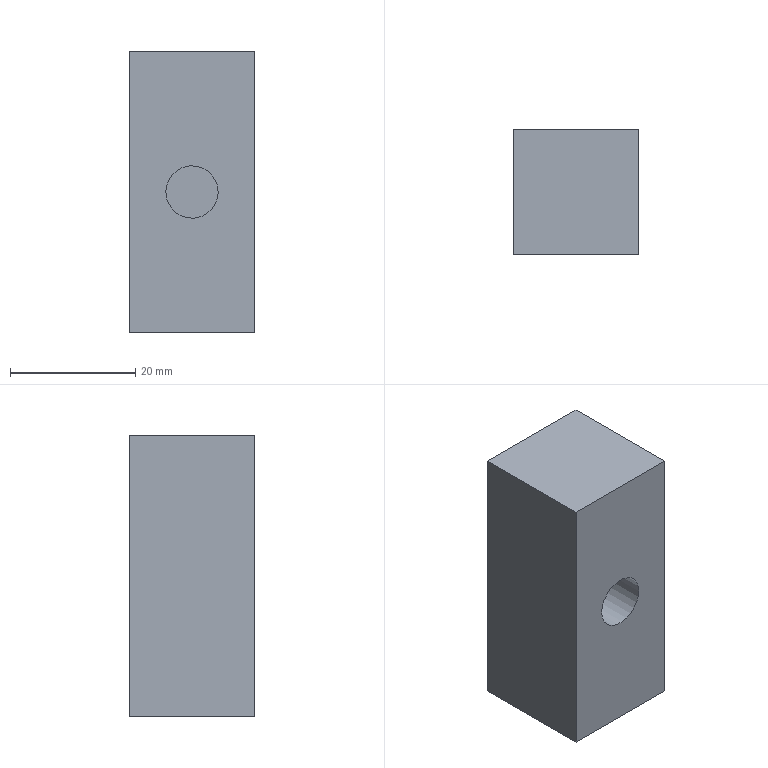Part | STEP file | SN10_017_001-02_BLOCO | 1 solid | 8 faces | box 20 x 20 x 45 mm | volume 17008 mm3 | plane 7 | cylinder 1 | commonest cylinder face diameters 8.376 x1
STEP:
#1=CARTESIAN_POINT('',(0.,0.,0.));
#2=DIRECTION('',(0.,0.,1.));
#3=DIRECTION('',(1.,0.,0.));
#4=AXIS2_PLACEMENT_3D('',#1,#2,#3);
#5=CARTESIAN_POINT('',(3876.675,-1747.,65.492));
#6=VERTEX_POINT('',#5);
#7=CARTESIAN_POINT('',(3873.,-1747.,67.5));
#8=DIRECTION('',(0.,1.,0.));
#9=DIRECTION('',(1.,0.,0.));
#10=AXIS2_PLACEMENT_3D('',#7,#8,#9);
#11=CIRCLE('',#10,4.188);
#12=CARTESIAN_POINT('',(3873.,-1747.,67.5));
#13=DIRECTION('',(0.,1.,0.));
#14=DIRECTION('',(0.,0.,1.));
#15=AXIS2_PLACEMENT_3D('',#12,#13,#14);
#16=PLANE('',#15);
#17=CARTESIAN_POINT('',(0.,0.));
#18=DIRECTION('',(0.,1.));
#19=AXIS2_PLACEMENT_2D('',#17,#18);
#20=CIRCLE('',#19,4.188);
#21=(GEOMETRIC_REPRESENTATION_CONTEXT(2)PARAMETRIC_REPRESENTATION_CONTEXT()REPRESENTATION_CONTEXT('',''));
#22=DEFINITIONAL_REPRESENTATION('',(#20),#21);
#23=PCURVE('',#16,#22);
#24=CARTESIAN_POINT('',(3873.,-1764.9,67.5));
#25=DIRECTION('',(0.,1.,0.));
#26=DIRECTION('',(0.8776,0.,-0.4794));
#27=AXIS2_PLACEMENT_3D('',#24,#25,#26);
#28=CYLINDRICAL_SURFACE('',#27,4.188);
#29=CARTESIAN_POINT('',(-0.5,17.9));
#30=DIRECTION('',(1.,0.));
#31=VECTOR('',#30,1.);
#32=LINE('',#29,#31);
#33=(GEOMETRIC_REPRESENTATION_CONTEXT(2)PARAMETRIC_REPRESENTATION_CONTEXT()REPRESENTATION_CONTEXT('',''));
#34=DEFINITIONAL_REPRESENTATION('',(#32),#33);
#35=PCURVE('',#28,#34);
#36=SURFACE_CURVE('',#11,(#23,#35),.PCURVE_S1.);
#37=EDGE_CURVE('',#6,#6,#36,.T.);
#38=ORIENTED_EDGE('',*,*,#37,.F.);
#39=EDGE_LOOP('',(#38));
#40=FACE_BOUND('',#39,.T.);
#41=ADVANCED_FACE('',(#40),#16,.F.);
#42=CARTESIAN_POINT('',(3883.,-1745.,90.));
#43=VERTEX_POINT('',#42);
#44=CARTESIAN_POINT('',(3863.,-1745.,90.));
#45=VERTEX_POINT('',#44);
#46=CARTESIAN_POINT('',(3883.,-1745.,90.));
#47=DIRECTION('',(-1.,0.,0.));
#48=VECTOR('',#47,1.);
#49=LINE('',#46,#48);
#50=CARTESIAN_POINT('',(0.,-1745.,0.));
#51=DIRECTION('',(0.,1.,0.));
#52=DIRECTION('',(0.,0.,1.));
#53=AXIS2_PLACEMENT_3D('',#50,#51,#52);
#54=PLANE('',#53);
#55=CARTESIAN_POINT('',(90.,3883.));
#56=DIRECTION('',(0.,-1.));
#57=VECTOR('',#56,1.);
#58=LINE('',#55,#57);
#59=(GEOMETRIC_REPRESENTATION_CONTEXT(2)PARAMETRIC_REPRESENTATION_CONTEXT()REPRESENTATION_CONTEXT('',''));
#60=DEFINITIONAL_REPRESENTATION('',(#58),#59);
#61=PCURVE('',#54,#60);
#62=CARTESIAN_POINT('',(3883.,-1745.,90.));
#63=DIRECTION('',(0.,0.,1.));
#64=DIRECTION('',(1.,0.,0.));
#65=AXIS2_PLACEMENT_3D('',#62,#63,#64);
#66=PLANE('',#65);
#67=CARTESIAN_POINT('',(0.,0.));
#68=DIRECTION('',(-1.,0.));
#69=VECTOR('',#68,1.);
#70=LINE('',#67,#69);
#71=(GEOMETRIC_REPRESENTATION_CONTEXT(2)PARAMETRIC_REPRESENTATION_CONTEXT()REPRESENTATION_CONTEXT('',''));
#72=DEFINITIONAL_REPRESENTATION('',(#70),#71);
#73=PCURVE('',#66,#72);
#74=SURFACE_CURVE('',#49,(#61,#73),.PCURVE_S1.);
#75=EDGE_CURVE('',#43,#45,#74,.T.);
#76=ORIENTED_EDGE('',*,*,#75,.F.);
#77=CARTESIAN_POINT('',(3883.,-1745.,45.));
#78=VERTEX_POINT('',#77);
#79=CARTESIAN_POINT('',(3883.,-1745.,45.));
#80=DIRECTION('',(0.,0.,1.));
#81=VECTOR('',#80,1.);
#82=LINE('',#79,#81);
#83=CARTESIAN_POINT('',(45.,3883.));
#84=DIRECTION('',(1.,0.));
#85=VECTOR('',#84,1.);
#86=LINE('',#83,#85);
#87=(GEOMETRIC_REPRESENTATION_CONTEXT(2)PARAMETRIC_REPRESENTATION_CONTEXT()REPRESENTATION_CONTEXT('',''));
#88=DEFINITIONAL_REPRESENTATION('',(#86),#87);
#89=PCURVE('',#54,#88);
#90=CARTESIAN_POINT('',(3883.,-1745.,45.));
#91=DIRECTION('',(1.,0.,0.));
#92=DIRECTION('',(0.,0.,-1.));
#93=AXIS2_PLACEMENT_3D('',#90,#91,#92);
#94=PLANE('',#93);
#95=CARTESIAN_POINT('',(0.,0.));
#96=DIRECTION('',(-1.,0.));
#97=VECTOR('',#96,1.);
#98=LINE('',#95,#97);
#99=(GEOMETRIC_REPRESENTATION_CONTEXT(2)PARAMETRIC_REPRESENTATION_CONTEXT()REPRESENTATION_CONTEXT('',''));
#100=DEFINITIONAL_REPRESENTATION('',(#98),#99);
#101=PCURVE('',#94,#100);
#102=SURFACE_CURVE('',#82,(#89,#101),.PCURVE_S1.);
#103=EDGE_CURVE('',#78,#43,#102,.T.);
#104=ORIENTED_EDGE('',*,*,#103,.F.);
#105=CARTESIAN_POINT('',(3863.,-1745.,45.));
#106=VERTEX_POINT('',#105);
#107=CARTESIAN_POINT('',(3863.,-1745.,45.));
#108=DIRECTION('',(1.,0.,0.));
#109=VECTOR('',#108,1.);
#110=LINE('',#107,#109);
#111=CARTESIAN_POINT('',(45.,3863.));
#112=DIRECTION('',(0.,1.));
#113=VECTOR('',#112,1.);
#114=LINE('',#111,#113);
#115=(GEOMETRIC_REPRESENTATION_CONTEXT(2)PARAMETRIC_REPRESENTATION_CONTEXT()REPRESENTATION_CONTEXT('',''));
#116=DEFINITIONAL_REPRESENTATION('',(#114),#115);
#117=PCURVE('',#54,#116);
#118=CARTESIAN_POINT('',(3863.,-1745.,45.));
#119=DIRECTION('',(0.,0.,-1.));
#120=DIRECTION('',(-1.,0.,0.));
#121=AXIS2_PLACEMENT_3D('',#118,#119,#120);
#122=PLANE('',#121);
#123=CARTESIAN_POINT('',(0.,0.));
#124=DIRECTION('',(-1.,0.));
#125=VECTOR('',#124,1.);
#126=LINE('',#123,#125);
#127=(GEOMETRIC_REPRESENTATION_CONTEXT(2)PARAMETRIC_REPRESENTATION_CONTEXT()REPRESENTATION_CONTEXT('',''));
#128=DEFINITIONAL_REPRESENTATION('',(#126),#127);
#129=PCURVE('',#122,#128);
#130=SURFACE_CURVE('',#110,(#117,#129),.PCURVE_S1.);
#131=EDGE_CURVE('',#106,#78,#130,.T.);
#132=ORIENTED_EDGE('',*,*,#131,.F.);
#133=CARTESIAN_POINT('',(3863.,-1745.,90.));
#134=DIRECTION('',(0.,0.,-1.));
#135=VECTOR('',#134,1.);
#136=LINE('',#133,#135);
#137=CARTESIAN_POINT('',(90.,3863.));
#138=DIRECTION('',(-1.,0.));
#139=VECTOR('',#138,1.);
#140=LINE('',#137,#139);
#141=(GEOMETRIC_REPRESENTATION_CONTEXT(2)PARAMETRIC_REPRESENTATION_CONTEXT()REPRESENTATION_CONTEXT('',''));
#142=DEFINITIONAL_REPRESENTATION('',(#140),#141);
#143=PCURVE('',#54,#142);
#144=CARTESIAN_POINT('',(3863.,-1745.,90.));
#145=DIRECTION('',(-1.,0.,0.));
#146=DIRECTION('',(0.,0.,1.));
#147=AXIS2_PLACEMENT_3D('',#144,#145,#146);
#148=PLANE('',#147);
#149=CARTESIAN_POINT('',(0.,0.));
#150=DIRECTION('',(-1.,0.));
#151=VECTOR('',#150,1.);
#152=LINE('',#149,#151);
#153=(GEOMETRIC_REPRESENTATION_CONTEXT(2)PARAMETRIC_REPRESENTATION_CONTEXT()REPRESENTATION_CONTEXT('',''));
#154=DEFINITIONAL_REPRESENTATION('',(#152),#153);
#155=PCURVE('',#148,#154);
#156=SURFACE_CURVE('',#136,(#143,#155),.PCURVE_S1.);
#157=EDGE_CURVE('',#45,#106,#156,.T.);
#158=ORIENTED_EDGE('',*,*,#157,.F.);
#159=EDGE_LOOP('',(#76,#104,#132,#158));
#160=FACE_BOUND('',#159,.T.);
#161=ADVANCED_FACE('',(#160),#54,.T.);
#162=CARTESIAN_POINT('',(3863.,-1765.,90.));
#163=VERTEX_POINT('',#162);
#164=CARTESIAN_POINT('',(3863.,-1765.,45.));
#165=VERTEX_POINT('',#164);
#166=CARTESIAN_POINT('',(3863.,-1765.,90.));
#167=DIRECTION('',(0.,0.,-1.));
#168=VECTOR('',#167,1.);
#169=LINE('',#166,#168);
#170=CARTESIAN_POINT('',(0.,-20.));
#171=DIRECTION('',(-1.,0.));
#172=VECTOR('',#171,1.);
#173=LINE('',#170,#172);
#174=(GEOMETRIC_REPRESENTATION_CONTEXT(2)PARAMETRIC_REPRESENTATION_CONTEXT()REPRESENTATION_CONTEXT('',''));
#175=DEFINITIONAL_REPRESENTATION('',(#173),#174);
#176=PCURVE('',#148,#175);
#177=CARTESIAN_POINT('',(0.,-1765.,0.));
#178=DIRECTION('',(0.,1.,0.));
#179=DIRECTION('',(0.,0.,1.));
#180=AXIS2_PLACEMENT_3D('',#177,#178,#179);
#181=PLANE('',#180);
#182=CARTESIAN_POINT('',(90.,3863.));
#183=DIRECTION('',(-1.,0.));
#184=VECTOR('',#183,1.);
#185=LINE('',#182,#184);
#186=(GEOMETRIC_REPRESENTATION_CONTEXT(2)PARAMETRIC_REPRESENTATION_CONTEXT()REPRESENTATION_CONTEXT('',''));
#187=DEFINITIONAL_REPRESENTATION('',(#185),#186);
#188=PCURVE('',#181,#187);
#189=SURFACE_CURVE('',#169,(#176,#188),.PCURVE_S1.);
#190=EDGE_CURVE('',#163,#165,#189,.T.);
#191=ORIENTED_EDGE('',*,*,#190,.F.);
#192=CARTESIAN_POINT('',(3863.,-1745.,90.));
#193=DIRECTION('',(0.,-1.,0.));
#194=VECTOR('',#193,1.);
#195=LINE('',#192,#194);
#196=CARTESIAN_POINT('',(0.,0.));
#197=DIRECTION('',(0.,-1.));
#198=VECTOR('',#197,1.);
#199=LINE('',#196,#198);
#200=(GEOMETRIC_REPRESENTATION_CONTEXT(2)PARAMETRIC_REPRESENTATION_CONTEXT()REPRESENTATION_CONTEXT('',''));
#201=DEFINITIONAL_REPRESENTATION('',(#199),#200);
#202=PCURVE('',#148,#201);
#203=CARTESIAN_POINT('',(-20.,0.));
#204=DIRECTION('',(0.,-1.));
#205=VECTOR('',#204,1.);
#206=LINE('',#203,#205);
#207=(GEOMETRIC_REPRESENTATION_CONTEXT(2)PARAMETRIC_REPRESENTATION_CONTEXT()REPRESENTATION_CONTEXT('',''));
#208=DEFINITIONAL_REPRESENTATION('',(#206),#207);
#209=PCURVE('',#66,#208);
#210=SURFACE_CURVE('',#195,(#202,#209),.PCURVE_S1.);
#211=EDGE_CURVE('',#45,#163,#210,.T.);
#212=ORIENTED_EDGE('',*,*,#211,.F.);
#213=ORIENTED_EDGE('',*,*,#157,.T.);
#214=CARTESIAN_POINT('',(3863.,-1745.,45.));
#215=DIRECTION('',(0.,-1.,0.));
#216=VECTOR('',#215,1.);
#217=LINE('',#214,#216);
#218=CARTESIAN_POINT('',(-45.,0.));
#219=DIRECTION('',(0.,-1.));
#220=VECTOR('',#219,1.);
#221=LINE('',#218,#220);
#222=(GEOMETRIC_REPRESENTATION_CONTEXT(2)PARAMETRIC_REPRESENTATION_CONTEXT()REPRESENTATION_CONTEXT('',''));
#223=DEFINITIONAL_REPRESENTATION('',(#221),#222);
#224=PCURVE('',#148,#223);
#225=CARTESIAN_POINT('',(0.,0.));
#226=DIRECTION('',(0.,-1.));
#227=VECTOR('',#226,1.);
#228=LINE('',#225,#227);
#229=(GEOMETRIC_REPRESENTATION_CONTEXT(2)PARAMETRIC_REPRESENTATION_CONTEXT()REPRESENTATION_CONTEXT('',''));
#230=DEFINITIONAL_REPRESENTATION('',(#228),#229);
#231=PCURVE('',#122,#230);
#232=SURFACE_CURVE('',#217,(#224,#231),.PCURVE_S1.);
#233=EDGE_CURVE('',#106,#165,#232,.T.);
#234=ORIENTED_EDGE('',*,*,#233,.T.);
#235=EDGE_LOOP('',(#191,#212,#213,#234));
#236=FACE_BOUND('',#235,.T.);
#237=ADVANCED_FACE('',(#236),#148,.T.);
#238=CARTESIAN_POINT('',(3883.,-1765.,45.));
#239=VERTEX_POINT('',#238);
#240=CARTESIAN_POINT('',(3863.,-1765.,45.));
#241=DIRECTION('',(1.,0.,0.));
#242=VECTOR('',#241,1.);
#243=LINE('',#240,#242);
#244=CARTESIAN_POINT('',(0.,-20.));
#245=DIRECTION('',(-1.,0.));
#246=VECTOR('',#245,1.);
#247=LINE('',#244,#246);
#248=(GEOMETRIC_REPRESENTATION_CONTEXT(2)PARAMETRIC_REPRESENTATION_CONTEXT()REPRESENTATION_CONTEXT('',''));
#249=DEFINITIONAL_REPRESENTATION('',(#247),#248);
#250=PCURVE('',#122,#249);
#251=CARTESIAN_POINT('',(45.,3863.));
#252=DIRECTION('',(0.,1.));
#253=VECTOR('',#252,1.);
#254=LINE('',#251,#253);
#255=(GEOMETRIC_REPRESENTATION_CONTEXT(2)PARAMETRIC_REPRESENTATION_CONTEXT()REPRESENTATION_CONTEXT('',''));
#256=DEFINITIONAL_REPRESENTATION('',(#254),#255);
#257=PCURVE('',#181,#256);
#258=SURFACE_CURVE('',#243,(#250,#257),.PCURVE_S1.);
#259=EDGE_CURVE('',#165,#239,#258,.T.);
#260=ORIENTED_EDGE('',*,*,#259,.F.);
#261=ORIENTED_EDGE('',*,*,#233,.F.);
#262=ORIENTED_EDGE('',*,*,#131,.T.);
#263=CARTESIAN_POINT('',(3883.,-1745.,45.));
#264=DIRECTION('',(0.,-1.,0.));
#265=VECTOR('',#264,1.);
#266=LINE('',#263,#265);
#267=CARTESIAN_POINT('',(-20.,0.));
#268=DIRECTION('',(0.,-1.));
#269=VECTOR('',#268,1.);
#270=LINE('',#267,#269);
#271=(GEOMETRIC_REPRESENTATION_CONTEXT(2)PARAMETRIC_REPRESENTATION_CONTEXT()REPRESENTATION_CONTEXT('',''));
#272=DEFINITIONAL_REPRESENTATION('',(#270),#271);
#273=PCURVE('',#122,#272);
#274=CARTESIAN_POINT('',(0.,0.));
#275=DIRECTION('',(0.,-1.));
#276=VECTOR('',#275,1.);
#277=LINE('',#274,#276);
#278=(GEOMETRIC_REPRESENTATION_CONTEXT(2)PARAMETRIC_REPRESENTATION_CONTEXT()REPRESENTATION_CONTEXT('',''));
#279=DEFINITIONAL_REPRESENTATION('',(#277),#278);
#280=PCURVE('',#94,#279);
#281=SURFACE_CURVE('',#266,(#273,#280),.PCURVE_S1.);
#282=EDGE_CURVE('',#78,#239,#281,.T.);
#283=ORIENTED_EDGE('',*,*,#282,.T.);
#284=EDGE_LOOP('',(#260,#261,#262,#283));
#285=FACE_BOUND('',#284,.T.);
#286=ADVANCED_FACE('',(#285),#122,.T.);
#287=CARTESIAN_POINT('',(3883.,-1765.,90.));
#288=VERTEX_POINT('',#287);
#289=CARTESIAN_POINT('',(3883.,-1765.,45.));
#290=DIRECTION('',(0.,0.,1.));
#291=VECTOR('',#290,1.);
#292=LINE('',#289,#291);
#293=CARTESIAN_POINT('',(0.,-20.));
#294=DIRECTION('',(-1.,0.));
#295=VECTOR('',#294,1.);
#296=LINE('',#293,#295);
#297=(GEOMETRIC_REPRESENTATION_CONTEXT(2)PARAMETRIC_REPRESENTATION_CONTEXT()REPRESENTATION_CONTEXT('',''));
#298=DEFINITIONAL_REPRESENTATION('',(#296),#297);
#299=PCURVE('',#94,#298);
#300=CARTESIAN_POINT('',(45.,3883.));
#301=DIRECTION('',(1.,0.));
#302=VECTOR('',#301,1.);
#303=LINE('',#300,#302);
#304=(GEOMETRIC_REPRESENTATION_CONTEXT(2)PARAMETRIC_REPRESENTATION_CONTEXT()REPRESENTATION_CONTEXT('',''));
#305=DEFINITIONAL_REPRESENTATION('',(#303),#304);
#306=PCURVE('',#181,#305);
#307=SURFACE_CURVE('',#292,(#299,#306),.PCURVE_S1.);
#308=EDGE_CURVE('',#239,#288,#307,.T.);
#309=ORIENTED_EDGE('',*,*,#308,.F.);
#310=ORIENTED_EDGE('',*,*,#282,.F.);
#311=ORIENTED_EDGE('',*,*,#103,.T.);
#312=CARTESIAN_POINT('',(3883.,-1745.,90.));
#313=DIRECTION('',(0.,-1.,0.));
#314=VECTOR('',#313,1.);
#315=LINE('',#312,#314);
#316=CARTESIAN_POINT('',(-45.,0.));
#317=DIRECTION('',(0.,-1.));
#318=VECTOR('',#317,1.);
#319=LINE('',#316,#318);
#320=(GEOMETRIC_REPRESENTATION_CONTEXT(2)PARAMETRIC_REPRESENTATION_CONTEXT()REPRESENTATION_CONTEXT('',''));
#321=DEFINITIONAL_REPRESENTATION('',(#319),#320);
#322=PCURVE('',#94,#321);
#323=CARTESIAN_POINT('',(0.,0.));
#324=DIRECTION('',(0.,-1.));
#325=VECTOR('',#324,1.);
#326=LINE('',#323,#325);
#327=(GEOMETRIC_REPRESENTATION_CONTEXT(2)PARAMETRIC_REPRESENTATION_CONTEXT()REPRESENTATION_CONTEXT('',''));
#328=DEFINITIONAL_REPRESENTATION('',(#326),#327);
#329=PCURVE('',#66,#328);
#330=SURFACE_CURVE('',#315,(#322,#329),.PCURVE_S1.);
#331=EDGE_CURVE('',#43,#288,#330,.T.);
#332=ORIENTED_EDGE('',*,*,#331,.T.);
#333=EDGE_LOOP('',(#309,#310,#311,#332));
#334=FACE_BOUND('',#333,.T.);
#335=ADVANCED_FACE('',(#334),#94,.T.);
#336=CARTESIAN_POINT('',(3883.,-1765.,90.));
#337=DIRECTION('',(-1.,0.,0.));
#338=VECTOR('',#337,1.);
#339=LINE('',#336,#338);
#340=CARTESIAN_POINT('',(0.,-20.));
#341=DIRECTION('',(-1.,0.));
#342=VECTOR('',#341,1.);
#343=LINE('',#340,#342);
#344=(GEOMETRIC_REPRESENTATION_CONTEXT(2)PARAMETRIC_REPRESENTATION_CONTEXT()REPRESENTATION_CONTEXT('',''));
#345=DEFINITIONAL_REPRESENTATION('',(#343),#344);
#346=PCURVE('',#66,#345);
#347=CARTESIAN_POINT('',(90.,3883.));
#348=DIRECTION('',(0.,-1.));
#349=VECTOR('',#348,1.);
#350=LINE('',#347,#349);
#351=(GEOMETRIC_REPRESENTATION_CONTEXT(2)PARAMETRIC_REPRESENTATION_CONTEXT()REPRESENTATION_CONTEXT('',''));
#352=DEFINITIONAL_REPRESENTATION('',(#350),#351);
#353=PCURVE('',#181,#352);
#354=SURFACE_CURVE('',#339,(#346,#353),.PCURVE_S1.);
#355=EDGE_CURVE('',#288,#163,#354,.T.);
#356=ORIENTED_EDGE('',*,*,#355,.F.);
#357=ORIENTED_EDGE('',*,*,#331,.F.);
#358=ORIENTED_EDGE('',*,*,#75,.T.);
#359=ORIENTED_EDGE('',*,*,#211,.T.);
#360=EDGE_LOOP('',(#356,#357,#358,#359));
#361=FACE_BOUND('',#360,.T.);
#362=ADVANCED_FACE('',(#361),#66,.T.);
#363=ORIENTED_EDGE('',*,*,#190,.T.);
#364=ORIENTED_EDGE('',*,*,#259,.T.);
#365=ORIENTED_EDGE('',*,*,#308,.T.);
#366=ORIENTED_EDGE('',*,*,#355,.T.);
#367=EDGE_LOOP('',(#363,#364,#365,#366));
#368=FACE_BOUND('',#367,.T.);
#369=CARTESIAN_POINT('',(3876.675,-1765.,65.492));
#370=VERTEX_POINT('',#369);
#371=CARTESIAN_POINT('',(3873.,-1765.,67.5));
#372=DIRECTION('',(0.,1.,0.));
#373=DIRECTION('',(1.,0.,0.));
#374=AXIS2_PLACEMENT_3D('',#371,#372,#373);
#375=CIRCLE('',#374,4.188);
#376=CARTESIAN_POINT('',(67.5,3873.));
#377=DIRECTION('',(0.,1.));
#378=AXIS2_PLACEMENT_2D('',#376,#377);
#379=CIRCLE('',#378,4.188);
#380=(GEOMETRIC_REPRESENTATION_CONTEXT(2)PARAMETRIC_REPRESENTATION_CONTEXT()REPRESENTATION_CONTEXT('',''));
#381=DEFINITIONAL_REPRESENTATION('',(#379),#380);
#382=PCURVE('',#181,#381);
#383=CARTESIAN_POINT('',(-0.5,-0.1));
#384=DIRECTION('',(1.,0.));
#385=VECTOR('',#384,1.);
#386=LINE('',#383,#385);
#387=(GEOMETRIC_REPRESENTATION_CONTEXT(2)PARAMETRIC_REPRESENTATION_CONTEXT()REPRESENTATION_CONTEXT('',''));
#388=DEFINITIONAL_REPRESENTATION('',(#386),#387);
#389=PCURVE('',#28,#388);
#390=SURFACE_CURVE('',#375,(#382,#389),.PCURVE_S1.);
#391=EDGE_CURVE('',#370,#370,#390,.T.);
#392=ORIENTED_EDGE('',*,*,#391,.T.);
#393=EDGE_LOOP('',(#392));
#394=FACE_BOUND('',#393,.T.);
#395=ADVANCED_FACE('',(#368,#394),#181,.F.);
#396=ORIENTED_EDGE('',*,*,#391,.T.);
#397=CARTESIAN_POINT('',(3876.675,-1765.,65.492));
#398=CARTESIAN_POINT('',(3876.675,-1747.,65.492));
#399=B_SPLINE_CURVE_WITH_KNOTS('',1,(#397,#398),.UNSPECIFIED.,.F.,.F.,(2,2),(-0.1,17.9),.PIECEWISE_BEZIER_KNOTS.);
#400=CARTESIAN_POINT('',(6.283,0.));
#401=DIRECTION('',(0.,1.));
#402=VECTOR('',#401,1.);
#403=LINE('',#400,#402);
#404=(GEOMETRIC_REPRESENTATION_CONTEXT(2)PARAMETRIC_REPRESENTATION_CONTEXT()REPRESENTATION_CONTEXT('',''));
#405=DEFINITIONAL_REPRESENTATION('',(#403),#404);
#406=PCURVE('',#28,#405);
#407=CARTESIAN_POINT('',(0.,0.));
#408=DIRECTION('',(0.,1.));
#409=VECTOR('',#408,1.);
#410=LINE('',#407,#409);
#411=(GEOMETRIC_REPRESENTATION_CONTEXT(2)PARAMETRIC_REPRESENTATION_CONTEXT()REPRESENTATION_CONTEXT('',''));
#412=DEFINITIONAL_REPRESENTATION('',(#410),#411);
#413=PCURVE('',#28,#412);
#414=SEAM_CURVE('',#399,(#406,#413),.PCURVE_S1.);
#415=EDGE_CURVE('',#370,#6,#414,.T.);
#416=ORIENTED_EDGE('',*,*,#415,.T.);
#417=ORIENTED_EDGE('',*,*,#37,.F.);
#418=ORIENTED_EDGE('',*,*,#415,.F.);
#419=EDGE_LOOP('',(#396,#416,#417,#418));
#420=FACE_BOUND('',#419,.F.);
#421=ADVANCED_FACE('',(#420),#28,.F.);
#422=CLOSED_SHELL('',(#41,#161,#237,#286,#335,#362,#395,#421));
#423=MANIFOLD_SOLID_BREP('',#422);
#424=(LENGTH_UNIT()NAMED_UNIT(*)SI_UNIT(.MILLI.,.METRE.));
#425=UNCERTAINTY_MEASURE_WITH_UNIT(LENGTH_MEASURE(0.000002),#424,'','');
#426=(NAMED_UNIT(*)PLANE_ANGLE_UNIT()SI_UNIT($,.RADIAN.));
#427=(NAMED_UNIT(*)SI_UNIT($,.STERADIAN.)SOLID_ANGLE_UNIT());
#428=(GEOMETRIC_REPRESENTATION_CONTEXT(3)GLOBAL_UNCERTAINTY_ASSIGNED_CONTEXT((#425))GLOBAL_UNIT_ASSIGNED_CONTEXT((#424,#426,#427))REPRESENTATION_CONTEXT('',''));
#429=ADVANCED_BREP_SHAPE_REPRESENTATION('',(#4,#423),#428);